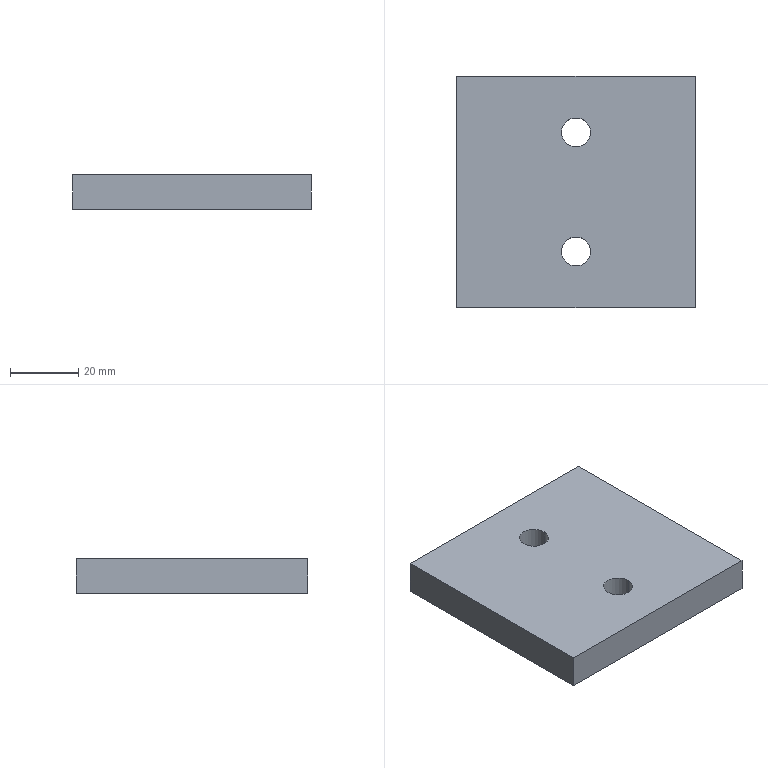Part | STEP file | BCC3 H12_13 | 1 solid | 10 faces | box 70 x 68 x 10 mm | volume 46465 mm3 | plane 6 | cylinder 4 | commonest cylinder face diameters 8.5 x4
STEP:
#1=CARTESIAN_POINT('',(0.,0.,0.));
#2=DIRECTION('',(0.,0.,1.));
#3=DIRECTION('',(1.,0.,0.));
#4=AXIS2_PLACEMENT_3D('',#1,#2,#3);
#5=CARTESIAN_POINT('',(-4.25,-17.5,10.));
#6=VERTEX_POINT('',#5);
#7=CARTESIAN_POINT('',(-4.25,-17.5,0.));
#8=VERTEX_POINT('',#7);
#9=CARTESIAN_POINT('',(-4.25,-17.5,10.));
#10=DIRECTION('',(0.,0.,-1.));
#11=VECTOR('',#10,1.);
#12=LINE('',#9,#11);
#13=CARTESIAN_POINT('',(0.,-17.5,10.));
#14=DIRECTION('',(0.,0.,-1.));
#15=DIRECTION('',(-1.,0.,0.));
#16=AXIS2_PLACEMENT_3D('',#13,#14,#15);
#17=CYLINDRICAL_SURFACE('',#16,4.25);
#18=CARTESIAN_POINT('',(6.283,0.));
#19=DIRECTION('',(0.,1.));
#20=VECTOR('',#19,1.);
#21=LINE('',#18,#20);
#22=(GEOMETRIC_REPRESENTATION_CONTEXT(2)PARAMETRIC_REPRESENTATION_CONTEXT()REPRESENTATION_CONTEXT('',''));
#23=DEFINITIONAL_REPRESENTATION('',(#21),#22);
#24=PCURVE('',#17,#23);
#25=CARTESIAN_POINT('',(0.,-17.5,10.));
#26=DIRECTION('',(0.,0.,-1.));
#27=DIRECTION('',(-1.,0.,0.));
#28=AXIS2_PLACEMENT_3D('',#25,#26,#27);
#29=CYLINDRICAL_SURFACE('',#28,4.25);
#30=CARTESIAN_POINT('',(0.,0.));
#31=DIRECTION('',(0.,1.));
#32=VECTOR('',#31,1.);
#33=LINE('',#30,#32);
#34=(GEOMETRIC_REPRESENTATION_CONTEXT(2)PARAMETRIC_REPRESENTATION_CONTEXT()REPRESENTATION_CONTEXT('',''));
#35=DEFINITIONAL_REPRESENTATION('',(#33),#34);
#36=PCURVE('',#29,#35);
#37=SURFACE_CURVE('',#12,(#24,#36),.PCURVE_S1.);
#38=EDGE_CURVE('',#6,#8,#37,.T.);
#39=ORIENTED_EDGE('',*,*,#38,.T.);
#40=CARTESIAN_POINT('',(4.25,-17.5,0.));
#41=VERTEX_POINT('',#40);
#42=CARTESIAN_POINT('',(0.,-17.5,0.));
#43=DIRECTION('',(0.,0.,1.));
#44=DIRECTION('',(1.,0.,0.));
#45=AXIS2_PLACEMENT_3D('',#42,#43,#44);
#46=CIRCLE('',#45,4.25);
#47=CARTESIAN_POINT('',(9.425,10.));
#48=DIRECTION('',(-1.,0.));
#49=VECTOR('',#48,1.);
#50=LINE('',#47,#49);
#51=(GEOMETRIC_REPRESENTATION_CONTEXT(2)PARAMETRIC_REPRESENTATION_CONTEXT()REPRESENTATION_CONTEXT('',''));
#52=DEFINITIONAL_REPRESENTATION('',(#50),#51);
#53=PCURVE('',#17,#52);
#54=CARTESIAN_POINT('',(0.,0.,0.));
#55=DIRECTION('',(0.,0.,1.));
#56=DIRECTION('',(1.,0.,0.));
#57=AXIS2_PLACEMENT_3D('',#54,#55,#56);
#58=PLANE('',#57);
#59=CARTESIAN_POINT('',(0.,-17.5));
#60=DIRECTION('',(1.,0.));
#61=AXIS2_PLACEMENT_2D('',#59,#60);
#62=CIRCLE('',#61,4.25);
#63=(GEOMETRIC_REPRESENTATION_CONTEXT(2)PARAMETRIC_REPRESENTATION_CONTEXT()REPRESENTATION_CONTEXT('',''));
#64=DEFINITIONAL_REPRESENTATION('',(#62),#63);
#65=PCURVE('',#58,#64);
#66=SURFACE_CURVE('',#46,(#53,#65),.PCURVE_S1.);
#67=EDGE_CURVE('',#8,#41,#66,.T.);
#68=ORIENTED_EDGE('',*,*,#67,.T.);
#69=CARTESIAN_POINT('',(4.25,-17.5,10.));
#70=VERTEX_POINT('',#69);
#71=CARTESIAN_POINT('',(4.25,-17.5,10.));
#72=DIRECTION('',(0.,0.,-1.));
#73=VECTOR('',#72,1.);
#74=LINE('',#71,#73);
#75=CARTESIAN_POINT('',(3.142,0.));
#76=DIRECTION('',(0.,1.));
#77=VECTOR('',#76,1.);
#78=LINE('',#75,#77);
#79=(GEOMETRIC_REPRESENTATION_CONTEXT(2)PARAMETRIC_REPRESENTATION_CONTEXT()REPRESENTATION_CONTEXT('',''));
#80=DEFINITIONAL_REPRESENTATION('',(#78),#79);
#81=PCURVE('',#17,#80);
#82=CARTESIAN_POINT('',(3.142,0.));
#83=DIRECTION('',(0.,1.));
#84=VECTOR('',#83,1.);
#85=LINE('',#82,#84);
#86=(GEOMETRIC_REPRESENTATION_CONTEXT(2)PARAMETRIC_REPRESENTATION_CONTEXT()REPRESENTATION_CONTEXT('',''));
#87=DEFINITIONAL_REPRESENTATION('',(#85),#86);
#88=PCURVE('',#29,#87);
#89=SURFACE_CURVE('',#74,(#81,#88),.PCURVE_S1.);
#90=EDGE_CURVE('',#70,#41,#89,.T.);
#91=ORIENTED_EDGE('',*,*,#90,.F.);
#92=CARTESIAN_POINT('',(0.,-17.5,10.));
#93=DIRECTION('',(0.,0.,1.));
#94=DIRECTION('',(1.,0.,0.));
#95=AXIS2_PLACEMENT_3D('',#92,#93,#94);
#96=CIRCLE('',#95,4.25);
#97=CARTESIAN_POINT('',(9.425,0.));
#98=DIRECTION('',(-1.,0.));
#99=VECTOR('',#98,1.);
#100=LINE('',#97,#99);
#101=(GEOMETRIC_REPRESENTATION_CONTEXT(2)PARAMETRIC_REPRESENTATION_CONTEXT()REPRESENTATION_CONTEXT('',''));
#102=DEFINITIONAL_REPRESENTATION('',(#100),#101);
#103=PCURVE('',#17,#102);
#104=CARTESIAN_POINT('',(0.,0.,10.));
#105=DIRECTION('',(0.,0.,1.));
#106=DIRECTION('',(1.,0.,0.));
#107=AXIS2_PLACEMENT_3D('',#104,#105,#106);
#108=PLANE('',#107);
#109=CARTESIAN_POINT('',(0.,-17.5));
#110=DIRECTION('',(1.,0.));
#111=AXIS2_PLACEMENT_2D('',#109,#110);
#112=CIRCLE('',#111,4.25);
#113=(GEOMETRIC_REPRESENTATION_CONTEXT(2)PARAMETRIC_REPRESENTATION_CONTEXT()REPRESENTATION_CONTEXT('',''));
#114=DEFINITIONAL_REPRESENTATION('',(#112),#113);
#115=PCURVE('',#108,#114);
#116=SURFACE_CURVE('',#96,(#103,#115),.PCURVE_S1.);
#117=EDGE_CURVE('',#6,#70,#116,.T.);
#118=ORIENTED_EDGE('',*,*,#117,.F.);
#119=EDGE_LOOP('',(#39,#68,#91,#118));
#120=FACE_BOUND('',#119,.F.);
#121=ADVANCED_FACE('',(#120),#17,.F.);
#122=CARTESIAN_POINT('',(-4.25,17.5,10.));
#123=VERTEX_POINT('',#122);
#124=CARTESIAN_POINT('',(-4.25,17.5,0.));
#125=VERTEX_POINT('',#124);
#126=CARTESIAN_POINT('',(-4.25,17.5,10.));
#127=DIRECTION('',(0.,0.,-1.));
#128=VECTOR('',#127,1.);
#129=LINE('',#126,#128);
#130=CARTESIAN_POINT('',(0.,17.5,10.));
#131=DIRECTION('',(0.,0.,-1.));
#132=DIRECTION('',(-1.,0.,0.));
#133=AXIS2_PLACEMENT_3D('',#130,#131,#132);
#134=CYLINDRICAL_SURFACE('',#133,4.25);
#135=CARTESIAN_POINT('',(6.283,0.));
#136=DIRECTION('',(0.,1.));
#137=VECTOR('',#136,1.);
#138=LINE('',#135,#137);
#139=(GEOMETRIC_REPRESENTATION_CONTEXT(2)PARAMETRIC_REPRESENTATION_CONTEXT()REPRESENTATION_CONTEXT('',''));
#140=DEFINITIONAL_REPRESENTATION('',(#138),#139);
#141=PCURVE('',#134,#140);
#142=CARTESIAN_POINT('',(0.,17.5,10.));
#143=DIRECTION('',(0.,0.,-1.));
#144=DIRECTION('',(-1.,0.,0.));
#145=AXIS2_PLACEMENT_3D('',#142,#143,#144);
#146=CYLINDRICAL_SURFACE('',#145,4.25);
#147=CARTESIAN_POINT('',(0.,0.));
#148=DIRECTION('',(0.,1.));
#149=VECTOR('',#148,1.);
#150=LINE('',#147,#149);
#151=(GEOMETRIC_REPRESENTATION_CONTEXT(2)PARAMETRIC_REPRESENTATION_CONTEXT()REPRESENTATION_CONTEXT('',''));
#152=DEFINITIONAL_REPRESENTATION('',(#150),#151);
#153=PCURVE('',#146,#152);
#154=SURFACE_CURVE('',#129,(#141,#153),.PCURVE_S1.);
#155=EDGE_CURVE('',#123,#125,#154,.T.);
#156=ORIENTED_EDGE('',*,*,#155,.T.);
#157=CARTESIAN_POINT('',(4.25,17.5,0.));
#158=VERTEX_POINT('',#157);
#159=CARTESIAN_POINT('',(0.,17.5,0.));
#160=DIRECTION('',(0.,0.,1.));
#161=DIRECTION('',(1.,0.,0.));
#162=AXIS2_PLACEMENT_3D('',#159,#160,#161);
#163=CIRCLE('',#162,4.25);
#164=CARTESIAN_POINT('',(9.425,10.));
#165=DIRECTION('',(-1.,0.));
#166=VECTOR('',#165,1.);
#167=LINE('',#164,#166);
#168=(GEOMETRIC_REPRESENTATION_CONTEXT(2)PARAMETRIC_REPRESENTATION_CONTEXT()REPRESENTATION_CONTEXT('',''));
#169=DEFINITIONAL_REPRESENTATION('',(#167),#168);
#170=PCURVE('',#134,#169);
#171=CARTESIAN_POINT('',(0.,17.5));
#172=DIRECTION('',(1.,0.));
#173=AXIS2_PLACEMENT_2D('',#171,#172);
#174=CIRCLE('',#173,4.25);
#175=(GEOMETRIC_REPRESENTATION_CONTEXT(2)PARAMETRIC_REPRESENTATION_CONTEXT()REPRESENTATION_CONTEXT('',''));
#176=DEFINITIONAL_REPRESENTATION('',(#174),#175);
#177=PCURVE('',#58,#176);
#178=SURFACE_CURVE('',#163,(#170,#177),.PCURVE_S1.);
#179=EDGE_CURVE('',#125,#158,#178,.T.);
#180=ORIENTED_EDGE('',*,*,#179,.T.);
#181=CARTESIAN_POINT('',(4.25,17.5,10.));
#182=VERTEX_POINT('',#181);
#183=CARTESIAN_POINT('',(4.25,17.5,10.));
#184=DIRECTION('',(0.,0.,-1.));
#185=VECTOR('',#184,1.);
#186=LINE('',#183,#185);
#187=CARTESIAN_POINT('',(3.142,0.));
#188=DIRECTION('',(0.,1.));
#189=VECTOR('',#188,1.);
#190=LINE('',#187,#189);
#191=(GEOMETRIC_REPRESENTATION_CONTEXT(2)PARAMETRIC_REPRESENTATION_CONTEXT()REPRESENTATION_CONTEXT('',''));
#192=DEFINITIONAL_REPRESENTATION('',(#190),#191);
#193=PCURVE('',#134,#192);
#194=CARTESIAN_POINT('',(3.142,0.));
#195=DIRECTION('',(0.,1.));
#196=VECTOR('',#195,1.);
#197=LINE('',#194,#196);
#198=(GEOMETRIC_REPRESENTATION_CONTEXT(2)PARAMETRIC_REPRESENTATION_CONTEXT()REPRESENTATION_CONTEXT('',''));
#199=DEFINITIONAL_REPRESENTATION('',(#197),#198);
#200=PCURVE('',#146,#199);
#201=SURFACE_CURVE('',#186,(#193,#200),.PCURVE_S1.);
#202=EDGE_CURVE('',#182,#158,#201,.T.);
#203=ORIENTED_EDGE('',*,*,#202,.F.);
#204=CARTESIAN_POINT('',(0.,17.5,10.));
#205=DIRECTION('',(0.,0.,1.));
#206=DIRECTION('',(1.,0.,0.));
#207=AXIS2_PLACEMENT_3D('',#204,#205,#206);
#208=CIRCLE('',#207,4.25);
#209=CARTESIAN_POINT('',(9.425,0.));
#210=DIRECTION('',(-1.,0.));
#211=VECTOR('',#210,1.);
#212=LINE('',#209,#211);
#213=(GEOMETRIC_REPRESENTATION_CONTEXT(2)PARAMETRIC_REPRESENTATION_CONTEXT()REPRESENTATION_CONTEXT('',''));
#214=DEFINITIONAL_REPRESENTATION('',(#212),#213);
#215=PCURVE('',#134,#214);
#216=CARTESIAN_POINT('',(0.,17.5));
#217=DIRECTION('',(1.,0.));
#218=AXIS2_PLACEMENT_2D('',#216,#217);
#219=CIRCLE('',#218,4.25);
#220=(GEOMETRIC_REPRESENTATION_CONTEXT(2)PARAMETRIC_REPRESENTATION_CONTEXT()REPRESENTATION_CONTEXT('',''));
#221=DEFINITIONAL_REPRESENTATION('',(#219),#220);
#222=PCURVE('',#108,#221);
#223=SURFACE_CURVE('',#208,(#215,#222),.PCURVE_S1.);
#224=EDGE_CURVE('',#123,#182,#223,.T.);
#225=ORIENTED_EDGE('',*,*,#224,.F.);
#226=EDGE_LOOP('',(#156,#180,#203,#225));
#227=FACE_BOUND('',#226,.F.);
#228=ADVANCED_FACE('',(#227),#134,.F.);
#229=ORIENTED_EDGE('',*,*,#224,.F.);
#230=CARTESIAN_POINT('',(0.,17.5,10.));
#231=DIRECTION('',(0.,0.,1.));
#232=DIRECTION('',(1.,0.,0.));
#233=AXIS2_PLACEMENT_3D('',#230,#231,#232);
#234=CIRCLE('',#233,4.25);
#235=CARTESIAN_POINT('',(0.,17.5));
#236=DIRECTION('',(1.,0.));
#237=AXIS2_PLACEMENT_2D('',#235,#236);
#238=CIRCLE('',#237,4.25);
#239=(GEOMETRIC_REPRESENTATION_CONTEXT(2)PARAMETRIC_REPRESENTATION_CONTEXT()REPRESENTATION_CONTEXT('',''));
#240=DEFINITIONAL_REPRESENTATION('',(#238),#239);
#241=PCURVE('',#108,#240);
#242=CARTESIAN_POINT('',(3.142,0.));
#243=DIRECTION('',(-1.,0.));
#244=VECTOR('',#243,1.);
#245=LINE('',#242,#244);
#246=(GEOMETRIC_REPRESENTATION_CONTEXT(2)PARAMETRIC_REPRESENTATION_CONTEXT()REPRESENTATION_CONTEXT('',''));
#247=DEFINITIONAL_REPRESENTATION('',(#245),#246);
#248=PCURVE('',#146,#247);
#249=SURFACE_CURVE('',#234,(#241,#248),.PCURVE_S1.);
#250=EDGE_CURVE('',#182,#123,#249,.T.);
#251=ORIENTED_EDGE('',*,*,#250,.F.);
#252=EDGE_LOOP('',(#229,#251));
#253=FACE_BOUND('',#252,.T.);
#254=CARTESIAN_POINT('',(-35.,34.,10.));
#255=VERTEX_POINT('',#254);
#256=CARTESIAN_POINT('',(-35.,-34.,10.));
#257=VERTEX_POINT('',#256);
#258=CARTESIAN_POINT('',(-35.,34.,10.));
#259=DIRECTION('',(0.,-1.,0.));
#260=VECTOR('',#259,1.);
#261=LINE('',#258,#260);
#262=CARTESIAN_POINT('',(-35.,34.));
#263=DIRECTION('',(0.,-1.));
#264=VECTOR('',#263,1.);
#265=LINE('',#262,#264);
#266=(GEOMETRIC_REPRESENTATION_CONTEXT(2)PARAMETRIC_REPRESENTATION_CONTEXT()REPRESENTATION_CONTEXT('',''));
#267=DEFINITIONAL_REPRESENTATION('',(#265),#266);
#268=PCURVE('',#108,#267);
#269=CARTESIAN_POINT('',(-35.,34.,10.));
#270=DIRECTION('',(1.,0.,0.));
#271=DIRECTION('',(0.,1.,0.));
#272=AXIS2_PLACEMENT_3D('',#269,#270,#271);
#273=PLANE('',#272);
#274=CARTESIAN_POINT('',(0.,0.));
#275=DIRECTION('',(-1.,0.));
#276=VECTOR('',#275,1.);
#277=LINE('',#274,#276);
#278=(GEOMETRIC_REPRESENTATION_CONTEXT(2)PARAMETRIC_REPRESENTATION_CONTEXT()REPRESENTATION_CONTEXT('',''));
#279=DEFINITIONAL_REPRESENTATION('',(#277),#278);
#280=PCURVE('',#273,#279);
#281=SURFACE_CURVE('',#261,(#268,#280),.PCURVE_S1.);
#282=EDGE_CURVE('',#255,#257,#281,.T.);
#283=ORIENTED_EDGE('',*,*,#282,.T.);
#284=CARTESIAN_POINT('',(35.,-34.,10.));
#285=VERTEX_POINT('',#284);
#286=CARTESIAN_POINT('',(-35.,-34.,10.));
#287=DIRECTION('',(1.,0.,0.));
#288=VECTOR('',#287,1.);
#289=LINE('',#286,#288);
#290=CARTESIAN_POINT('',(-35.,-34.));
#291=DIRECTION('',(1.,0.));
#292=VECTOR('',#291,1.);
#293=LINE('',#290,#292);
#294=(GEOMETRIC_REPRESENTATION_CONTEXT(2)PARAMETRIC_REPRESENTATION_CONTEXT()REPRESENTATION_CONTEXT('',''));
#295=DEFINITIONAL_REPRESENTATION('',(#293),#294);
#296=PCURVE('',#108,#295);
#297=CARTESIAN_POINT('',(-35.,-34.,10.));
#298=DIRECTION('',(0.,1.,0.));
#299=DIRECTION('',(0.,0.,1.));
#300=AXIS2_PLACEMENT_3D('',#297,#298,#299);
#301=PLANE('',#300);
#302=CARTESIAN_POINT('',(0.,0.));
#303=DIRECTION('',(0.,1.));
#304=VECTOR('',#303,1.);
#305=LINE('',#302,#304);
#306=(GEOMETRIC_REPRESENTATION_CONTEXT(2)PARAMETRIC_REPRESENTATION_CONTEXT()REPRESENTATION_CONTEXT('',''));
#307=DEFINITIONAL_REPRESENTATION('',(#305),#306);
#308=PCURVE('',#301,#307);
#309=SURFACE_CURVE('',#289,(#296,#308),.PCURVE_S1.);
#310=EDGE_CURVE('',#257,#285,#309,.T.);
#311=ORIENTED_EDGE('',*,*,#310,.T.);
#312=CARTESIAN_POINT('',(35.,34.,10.));
#313=VERTEX_POINT('',#312);
#314=CARTESIAN_POINT('',(35.,34.,10.));
#315=DIRECTION('',(0.,1.,0.));
#316=VECTOR('',#315,1.);
#317=LINE('',#314,#316);
#318=CARTESIAN_POINT('',(35.,34.));
#319=DIRECTION('',(0.,1.));
#320=VECTOR('',#319,1.);
#321=LINE('',#318,#320);
#322=(GEOMETRIC_REPRESENTATION_CONTEXT(2)PARAMETRIC_REPRESENTATION_CONTEXT()REPRESENTATION_CONTEXT('',''));
#323=DEFINITIONAL_REPRESENTATION('',(#321),#322);
#324=PCURVE('',#108,#323);
#325=CARTESIAN_POINT('',(35.,34.,10.));
#326=DIRECTION('',(-1.,0.,0.));
#327=DIRECTION('',(0.,-1.,0.));
#328=AXIS2_PLACEMENT_3D('',#325,#326,#327);
#329=PLANE('',#328);
#330=CARTESIAN_POINT('',(0.,0.));
#331=DIRECTION('',(-1.,0.));
#332=VECTOR('',#331,1.);
#333=LINE('',#330,#332);
#334=(GEOMETRIC_REPRESENTATION_CONTEXT(2)PARAMETRIC_REPRESENTATION_CONTEXT()REPRESENTATION_CONTEXT('',''));
#335=DEFINITIONAL_REPRESENTATION('',(#333),#334);
#336=PCURVE('',#329,#335);
#337=SURFACE_CURVE('',#317,(#324,#336),.PCURVE_S1.);
#338=EDGE_CURVE('',#285,#313,#337,.T.);
#339=ORIENTED_EDGE('',*,*,#338,.T.);
#340=CARTESIAN_POINT('',(-35.,34.,10.));
#341=DIRECTION('',(-1.,0.,0.));
#342=VECTOR('',#341,1.);
#343=LINE('',#340,#342);
#344=CARTESIAN_POINT('',(-35.,34.));
#345=DIRECTION('',(-1.,0.));
#346=VECTOR('',#345,1.);
#347=LINE('',#344,#346);
#348=(GEOMETRIC_REPRESENTATION_CONTEXT(2)PARAMETRIC_REPRESENTATION_CONTEXT()REPRESENTATION_CONTEXT('',''));
#349=DEFINITIONAL_REPRESENTATION('',(#347),#348);
#350=PCURVE('',#108,#349);
#351=CARTESIAN_POINT('',(-35.,34.,10.));
#352=DIRECTION('',(0.,-1.,0.));
#353=DIRECTION('',(1.,0.,0.));
#354=AXIS2_PLACEMENT_3D('',#351,#352,#353);
#355=PLANE('',#354);
#356=CARTESIAN_POINT('',(0.,0.));
#357=DIRECTION('',(-1.,0.));
#358=VECTOR('',#357,1.);
#359=LINE('',#356,#358);
#360=(GEOMETRIC_REPRESENTATION_CONTEXT(2)PARAMETRIC_REPRESENTATION_CONTEXT()REPRESENTATION_CONTEXT('',''));
#361=DEFINITIONAL_REPRESENTATION('',(#359),#360);
#362=PCURVE('',#355,#361);
#363=SURFACE_CURVE('',#343,(#350,#362),.PCURVE_S1.);
#364=EDGE_CURVE('',#313,#255,#363,.T.);
#365=ORIENTED_EDGE('',*,*,#364,.T.);
#366=EDGE_LOOP('',(#283,#311,#339,#365));
#367=FACE_BOUND('',#366,.T.);
#368=ORIENTED_EDGE('',*,*,#117,.F.);
#369=CARTESIAN_POINT('',(0.,-17.5,10.));
#370=DIRECTION('',(0.,0.,1.));
#371=DIRECTION('',(1.,0.,0.));
#372=AXIS2_PLACEMENT_3D('',#369,#370,#371);
#373=CIRCLE('',#372,4.25);
#374=CARTESIAN_POINT('',(0.,-17.5));
#375=DIRECTION('',(1.,0.));
#376=AXIS2_PLACEMENT_2D('',#374,#375);
#377=CIRCLE('',#376,4.25);
#378=(GEOMETRIC_REPRESENTATION_CONTEXT(2)PARAMETRIC_REPRESENTATION_CONTEXT()REPRESENTATION_CONTEXT('',''));
#379=DEFINITIONAL_REPRESENTATION('',(#377),#378);
#380=PCURVE('',#108,#379);
#381=CARTESIAN_POINT('',(3.142,0.));
#382=DIRECTION('',(-1.,0.));
#383=VECTOR('',#382,1.);
#384=LINE('',#381,#383);
#385=(GEOMETRIC_REPRESENTATION_CONTEXT(2)PARAMETRIC_REPRESENTATION_CONTEXT()REPRESENTATION_CONTEXT('',''));
#386=DEFINITIONAL_REPRESENTATION('',(#384),#385);
#387=PCURVE('',#29,#386);
#388=SURFACE_CURVE('',#373,(#380,#387),.PCURVE_S1.);
#389=EDGE_CURVE('',#70,#6,#388,.T.);
#390=ORIENTED_EDGE('',*,*,#389,.F.);
#391=EDGE_LOOP('',(#368,#390));
#392=FACE_BOUND('',#391,.T.);
#393=ADVANCED_FACE('',(#253,#367,#392),#108,.T.);
#394=ORIENTED_EDGE('',*,*,#179,.T.);
#395=CARTESIAN_POINT('',(0.,17.5,0.));
#396=DIRECTION('',(0.,0.,1.));
#397=DIRECTION('',(1.,0.,0.));
#398=AXIS2_PLACEMENT_3D('',#395,#396,#397);
#399=CIRCLE('',#398,4.25);
#400=CARTESIAN_POINT('',(0.,17.5));
#401=DIRECTION('',(1.,0.));
#402=AXIS2_PLACEMENT_2D('',#400,#401);
#403=CIRCLE('',#402,4.25);
#404=(GEOMETRIC_REPRESENTATION_CONTEXT(2)PARAMETRIC_REPRESENTATION_CONTEXT()REPRESENTATION_CONTEXT('',''));
#405=DEFINITIONAL_REPRESENTATION('',(#403),#404);
#406=PCURVE('',#58,#405);
#407=CARTESIAN_POINT('',(3.142,10.));
#408=DIRECTION('',(-1.,0.));
#409=VECTOR('',#408,1.);
#410=LINE('',#407,#409);
#411=(GEOMETRIC_REPRESENTATION_CONTEXT(2)PARAMETRIC_REPRESENTATION_CONTEXT()REPRESENTATION_CONTEXT('',''));
#412=DEFINITIONAL_REPRESENTATION('',(#410),#411);
#413=PCURVE('',#146,#412);
#414=SURFACE_CURVE('',#399,(#406,#413),.PCURVE_S1.);
#415=EDGE_CURVE('',#158,#125,#414,.T.);
#416=ORIENTED_EDGE('',*,*,#415,.T.);
#417=EDGE_LOOP('',(#394,#416));
#418=FACE_BOUND('',#417,.T.);
#419=CARTESIAN_POINT('',(-35.,34.,0.));
#420=VERTEX_POINT('',#419);
#421=CARTESIAN_POINT('',(-35.,-34.,0.));
#422=VERTEX_POINT('',#421);
#423=CARTESIAN_POINT('',(-35.,34.,0.));
#424=DIRECTION('',(0.,-1.,0.));
#425=VECTOR('',#424,1.);
#426=LINE('',#423,#425);
#427=CARTESIAN_POINT('',(-35.,34.));
#428=DIRECTION('',(0.,-1.));
#429=VECTOR('',#428,1.);
#430=LINE('',#427,#429);
#431=(GEOMETRIC_REPRESENTATION_CONTEXT(2)PARAMETRIC_REPRESENTATION_CONTEXT()REPRESENTATION_CONTEXT('',''));
#432=DEFINITIONAL_REPRESENTATION('',(#430),#431);
#433=PCURVE('',#58,#432);
#434=CARTESIAN_POINT('',(0.,-10.));
#435=DIRECTION('',(-1.,0.));
#436=VECTOR('',#435,1.);
#437=LINE('',#434,#436);
#438=(GEOMETRIC_REPRESENTATION_CONTEXT(2)PARAMETRIC_REPRESENTATION_CONTEXT()REPRESENTATION_CONTEXT('',''));
#439=DEFINITIONAL_REPRESENTATION('',(#437),#438);
#440=PCURVE('',#273,#439);
#441=SURFACE_CURVE('',#426,(#433,#440),.PCURVE_S1.);
#442=EDGE_CURVE('',#420,#422,#441,.T.);
#443=ORIENTED_EDGE('',*,*,#442,.F.);
#444=CARTESIAN_POINT('',(35.,34.,0.));
#445=VERTEX_POINT('',#444);
#446=CARTESIAN_POINT('',(-35.,34.,0.));
#447=DIRECTION('',(-1.,0.,0.));
#448=VECTOR('',#447,1.);
#449=LINE('',#446,#448);
#450=CARTESIAN_POINT('',(-35.,34.));
#451=DIRECTION('',(-1.,0.));
#452=VECTOR('',#451,1.);
#453=LINE('',#450,#452);
#454=(GEOMETRIC_REPRESENTATION_CONTEXT(2)PARAMETRIC_REPRESENTATION_CONTEXT()REPRESENTATION_CONTEXT('',''));
#455=DEFINITIONAL_REPRESENTATION('',(#453),#454);
#456=PCURVE('',#58,#455);
#457=CARTESIAN_POINT('',(0.,-10.));
#458=DIRECTION('',(-1.,0.));
#459=VECTOR('',#458,1.);
#460=LINE('',#457,#459);
#461=(GEOMETRIC_REPRESENTATION_CONTEXT(2)PARAMETRIC_REPRESENTATION_CONTEXT()REPRESENTATION_CONTEXT('',''));
#462=DEFINITIONAL_REPRESENTATION('',(#460),#461);
#463=PCURVE('',#355,#462);
#464=SURFACE_CURVE('',#449,(#456,#463),.PCURVE_S1.);
#465=EDGE_CURVE('',#445,#420,#464,.T.);
#466=ORIENTED_EDGE('',*,*,#465,.F.);
#467=CARTESIAN_POINT('',(35.,-34.,0.));
#468=VERTEX_POINT('',#467);
#469=CARTESIAN_POINT('',(35.,34.,0.));
#470=DIRECTION('',(0.,1.,0.));
#471=VECTOR('',#470,1.);
#472=LINE('',#469,#471);
#473=CARTESIAN_POINT('',(35.,34.));
#474=DIRECTION('',(0.,1.));
#475=VECTOR('',#474,1.);
#476=LINE('',#473,#475);
#477=(GEOMETRIC_REPRESENTATION_CONTEXT(2)PARAMETRIC_REPRESENTATION_CONTEXT()REPRESENTATION_CONTEXT('',''));
#478=DEFINITIONAL_REPRESENTATION('',(#476),#477);
#479=PCURVE('',#58,#478);
#480=CARTESIAN_POINT('',(0.,-10.));
#481=DIRECTION('',(-1.,0.));
#482=VECTOR('',#481,1.);
#483=LINE('',#480,#482);
#484=(GEOMETRIC_REPRESENTATION_CONTEXT(2)PARAMETRIC_REPRESENTATION_CONTEXT()REPRESENTATION_CONTEXT('',''));
#485=DEFINITIONAL_REPRESENTATION('',(#483),#484);
#486=PCURVE('',#329,#485);
#487=SURFACE_CURVE('',#472,(#479,#486),.PCURVE_S1.);
#488=EDGE_CURVE('',#468,#445,#487,.T.);
#489=ORIENTED_EDGE('',*,*,#488,.F.);
#490=CARTESIAN_POINT('',(-35.,-34.,0.));
#491=DIRECTION('',(1.,0.,0.));
#492=VECTOR('',#491,1.);
#493=LINE('',#490,#492);
#494=CARTESIAN_POINT('',(-35.,-34.));
#495=DIRECTION('',(1.,0.));
#496=VECTOR('',#495,1.);
#497=LINE('',#494,#496);
#498=(GEOMETRIC_REPRESENTATION_CONTEXT(2)PARAMETRIC_REPRESENTATION_CONTEXT()REPRESENTATION_CONTEXT('',''));
#499=DEFINITIONAL_REPRESENTATION('',(#497),#498);
#500=PCURVE('',#58,#499);
#501=CARTESIAN_POINT('',(-10.,0.));
#502=DIRECTION('',(0.,1.));
#503=VECTOR('',#502,1.);
#504=LINE('',#501,#503);
#505=(GEOMETRIC_REPRESENTATION_CONTEXT(2)PARAMETRIC_REPRESENTATION_CONTEXT()REPRESENTATION_CONTEXT('',''));
#506=DEFINITIONAL_REPRESENTATION('',(#504),#505);
#507=PCURVE('',#301,#506);
#508=SURFACE_CURVE('',#493,(#500,#507),.PCURVE_S1.);
#509=EDGE_CURVE('',#422,#468,#508,.T.);
#510=ORIENTED_EDGE('',*,*,#509,.F.);
#511=EDGE_LOOP('',(#443,#466,#489,#510));
#512=FACE_BOUND('',#511,.T.);
#513=ORIENTED_EDGE('',*,*,#67,.T.);
#514=CARTESIAN_POINT('',(0.,-17.5,0.));
#515=DIRECTION('',(0.,0.,1.));
#516=DIRECTION('',(1.,0.,0.));
#517=AXIS2_PLACEMENT_3D('',#514,#515,#516);
#518=CIRCLE('',#517,4.25);
#519=CARTESIAN_POINT('',(0.,-17.5));
#520=DIRECTION('',(1.,0.));
#521=AXIS2_PLACEMENT_2D('',#519,#520);
#522=CIRCLE('',#521,4.25);
#523=(GEOMETRIC_REPRESENTATION_CONTEXT(2)PARAMETRIC_REPRESENTATION_CONTEXT()REPRESENTATION_CONTEXT('',''));
#524=DEFINITIONAL_REPRESENTATION('',(#522),#523);
#525=PCURVE('',#58,#524);
#526=CARTESIAN_POINT('',(3.142,10.));
#527=DIRECTION('',(-1.,0.));
#528=VECTOR('',#527,1.);
#529=LINE('',#526,#528);
#530=(GEOMETRIC_REPRESENTATION_CONTEXT(2)PARAMETRIC_REPRESENTATION_CONTEXT()REPRESENTATION_CONTEXT('',''));
#531=DEFINITIONAL_REPRESENTATION('',(#529),#530);
#532=PCURVE('',#29,#531);
#533=SURFACE_CURVE('',#518,(#525,#532),.PCURVE_S1.);
#534=EDGE_CURVE('',#41,#8,#533,.T.);
#535=ORIENTED_EDGE('',*,*,#534,.T.);
#536=EDGE_LOOP('',(#513,#535));
#537=FACE_BOUND('',#536,.T.);
#538=ADVANCED_FACE('',(#418,#512,#537),#58,.F.);
#539=ORIENTED_EDGE('',*,*,#442,.T.);
#540=CARTESIAN_POINT('',(-35.,-34.,10.));
#541=DIRECTION('',(0.,0.,-1.));
#542=VECTOR('',#541,1.);
#543=LINE('',#540,#542);
#544=CARTESIAN_POINT('',(-68.,0.));
#545=DIRECTION('',(0.,-1.));
#546=VECTOR('',#545,1.);
#547=LINE('',#544,#546);
#548=(GEOMETRIC_REPRESENTATION_CONTEXT(2)PARAMETRIC_REPRESENTATION_CONTEXT()REPRESENTATION_CONTEXT('',''));
#549=DEFINITIONAL_REPRESENTATION('',(#547),#548);
#550=PCURVE('',#273,#549);
#551=CARTESIAN_POINT('',(0.,0.));
#552=DIRECTION('',(-1.,0.));
#553=VECTOR('',#552,1.);
#554=LINE('',#551,#553);
#555=(GEOMETRIC_REPRESENTATION_CONTEXT(2)PARAMETRIC_REPRESENTATION_CONTEXT()REPRESENTATION_CONTEXT('',''));
#556=DEFINITIONAL_REPRESENTATION('',(#554),#555);
#557=PCURVE('',#301,#556);
#558=SURFACE_CURVE('',#543,(#550,#557),.PCURVE_S1.);
#559=EDGE_CURVE('',#257,#422,#558,.T.);
#560=ORIENTED_EDGE('',*,*,#559,.F.);
#561=ORIENTED_EDGE('',*,*,#282,.F.);
#562=CARTESIAN_POINT('',(-35.,34.,10.));
#563=DIRECTION('',(0.,0.,-1.));
#564=VECTOR('',#563,1.);
#565=LINE('',#562,#564);
#566=CARTESIAN_POINT('',(0.,0.));
#567=DIRECTION('',(0.,-1.));
#568=VECTOR('',#567,1.);
#569=LINE('',#566,#568);
#570=(GEOMETRIC_REPRESENTATION_CONTEXT(2)PARAMETRIC_REPRESENTATION_CONTEXT()REPRESENTATION_CONTEXT('',''));
#571=DEFINITIONAL_REPRESENTATION('',(#569),#570);
#572=PCURVE('',#273,#571);
#573=CARTESIAN_POINT('',(0.,0.));
#574=DIRECTION('',(0.,-1.));
#575=VECTOR('',#574,1.);
#576=LINE('',#573,#575);
#577=(GEOMETRIC_REPRESENTATION_CONTEXT(2)PARAMETRIC_REPRESENTATION_CONTEXT()REPRESENTATION_CONTEXT('',''));
#578=DEFINITIONAL_REPRESENTATION('',(#576),#577);
#579=PCURVE('',#355,#578);
#580=SURFACE_CURVE('',#565,(#572,#579),.PCURVE_S1.);
#581=EDGE_CURVE('',#255,#420,#580,.T.);
#582=ORIENTED_EDGE('',*,*,#581,.T.);
#583=EDGE_LOOP('',(#539,#560,#561,#582));
#584=FACE_BOUND('',#583,.T.);
#585=ADVANCED_FACE('',(#584),#273,.F.);
#586=ORIENTED_EDGE('',*,*,#509,.T.);
#587=CARTESIAN_POINT('',(35.,-34.,10.));
#588=DIRECTION('',(0.,0.,-1.));
#589=VECTOR('',#588,1.);
#590=LINE('',#587,#589);
#591=CARTESIAN_POINT('',(0.,70.));
#592=DIRECTION('',(-1.,0.));
#593=VECTOR('',#592,1.);
#594=LINE('',#591,#593);
#595=(GEOMETRIC_REPRESENTATION_CONTEXT(2)PARAMETRIC_REPRESENTATION_CONTEXT()REPRESENTATION_CONTEXT('',''));
#596=DEFINITIONAL_REPRESENTATION('',(#594),#595);
#597=PCURVE('',#301,#596);
#598=CARTESIAN_POINT('',(68.,0.));
#599=DIRECTION('',(0.,-1.));
#600=VECTOR('',#599,1.);
#601=LINE('',#598,#600);
#602=(GEOMETRIC_REPRESENTATION_CONTEXT(2)PARAMETRIC_REPRESENTATION_CONTEXT()REPRESENTATION_CONTEXT('',''));
#603=DEFINITIONAL_REPRESENTATION('',(#601),#602);
#604=PCURVE('',#329,#603);
#605=SURFACE_CURVE('',#590,(#597,#604),.PCURVE_S1.);
#606=EDGE_CURVE('',#285,#468,#605,.T.);
#607=ORIENTED_EDGE('',*,*,#606,.F.);
#608=ORIENTED_EDGE('',*,*,#310,.F.);
#609=ORIENTED_EDGE('',*,*,#559,.T.);
#610=EDGE_LOOP('',(#586,#607,#608,#609));
#611=FACE_BOUND('',#610,.T.);
#612=ADVANCED_FACE('',(#611),#301,.F.);
#613=ORIENTED_EDGE('',*,*,#488,.T.);
#614=CARTESIAN_POINT('',(35.,34.,10.));
#615=DIRECTION('',(0.,0.,-1.));
#616=VECTOR('',#615,1.);
#617=LINE('',#614,#616);
#618=CARTESIAN_POINT('',(0.,0.));
#619=DIRECTION('',(0.,-1.));
#620=VECTOR('',#619,1.);
#621=LINE('',#618,#620);
#622=(GEOMETRIC_REPRESENTATION_CONTEXT(2)PARAMETRIC_REPRESENTATION_CONTEXT()REPRESENTATION_CONTEXT('',''));
#623=DEFINITIONAL_REPRESENTATION('',(#621),#622);
#624=PCURVE('',#329,#623);
#625=CARTESIAN_POINT('',(70.,0.));
#626=DIRECTION('',(0.,-1.));
#627=VECTOR('',#626,1.);
#628=LINE('',#625,#627);
#629=(GEOMETRIC_REPRESENTATION_CONTEXT(2)PARAMETRIC_REPRESENTATION_CONTEXT()REPRESENTATION_CONTEXT('',''));
#630=DEFINITIONAL_REPRESENTATION('',(#628),#629);
#631=PCURVE('',#355,#630);
#632=SURFACE_CURVE('',#617,(#624,#631),.PCURVE_S1.);
#633=EDGE_CURVE('',#313,#445,#632,.T.);
#634=ORIENTED_EDGE('',*,*,#633,.F.);
#635=ORIENTED_EDGE('',*,*,#338,.F.);
#636=ORIENTED_EDGE('',*,*,#606,.T.);
#637=EDGE_LOOP('',(#613,#634,#635,#636));
#638=FACE_BOUND('',#637,.T.);
#639=ADVANCED_FACE('',(#638),#329,.F.);
#640=ORIENTED_EDGE('',*,*,#465,.T.);
#641=ORIENTED_EDGE('',*,*,#581,.F.);
#642=ORIENTED_EDGE('',*,*,#364,.F.);
#643=ORIENTED_EDGE('',*,*,#633,.T.);
#644=EDGE_LOOP('',(#640,#641,#642,#643));
#645=FACE_BOUND('',#644,.T.);
#646=ADVANCED_FACE('',(#645),#355,.F.);
#647=ORIENTED_EDGE('',*,*,#415,.T.);
#648=ORIENTED_EDGE('',*,*,#155,.F.);
#649=ORIENTED_EDGE('',*,*,#250,.F.);
#650=ORIENTED_EDGE('',*,*,#202,.T.);
#651=EDGE_LOOP('',(#647,#648,#649,#650));
#652=FACE_BOUND('',#651,.F.);
#653=ADVANCED_FACE('',(#652),#146,.F.);
#654=ORIENTED_EDGE('',*,*,#534,.T.);
#655=ORIENTED_EDGE('',*,*,#38,.F.);
#656=ORIENTED_EDGE('',*,*,#389,.F.);
#657=ORIENTED_EDGE('',*,*,#90,.T.);
#658=EDGE_LOOP('',(#654,#655,#656,#657));
#659=FACE_BOUND('',#658,.F.);
#660=ADVANCED_FACE('',(#659),#29,.F.);
#661=CLOSED_SHELL('',(#121,#228,#393,#538,#585,#612,#639,#646,#653,#660));
#662=MANIFOLD_SOLID_BREP('',#661);
#663=(LENGTH_UNIT()NAMED_UNIT(*)SI_UNIT(.MILLI.,.METRE.));
#664=UNCERTAINTY_MEASURE_WITH_UNIT(LENGTH_MEASURE(0.0000001),#663,'','');
#665=(NAMED_UNIT(*)PLANE_ANGLE_UNIT()SI_UNIT($,.RADIAN.));
#666=(NAMED_UNIT(*)SI_UNIT($,.STERADIAN.)SOLID_ANGLE_UNIT());
#667=(GEOMETRIC_REPRESENTATION_CONTEXT(3)GLOBAL_UNCERTAINTY_ASSIGNED_CONTEXT((#664))GLOBAL_UNIT_ASSIGNED_CONTEXT((#663,#665,#666))REPRESENTATION_CONTEXT('',''));
#668=ADVANCED_BREP_SHAPE_REPRESENTATION('',(#4,#662),#667);